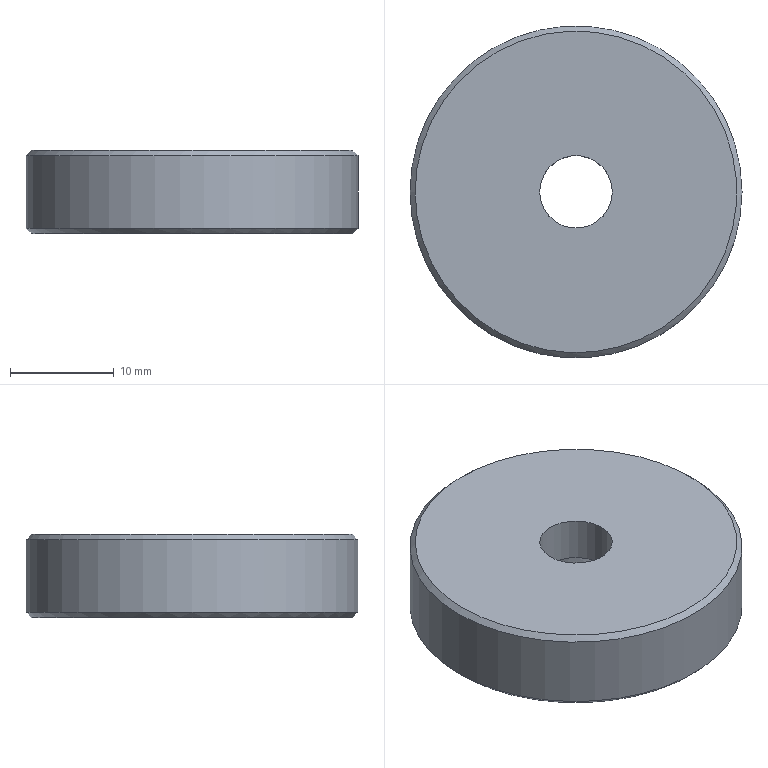Part | STEP file | solid 28 | 1 solid | 7 faces | box 32 x 32 x 8 mm | volume 5898 mm3 | cone 3 | plane 2 | cylinder 2 | commonest cylinder face diameters 7 x1 32 x1